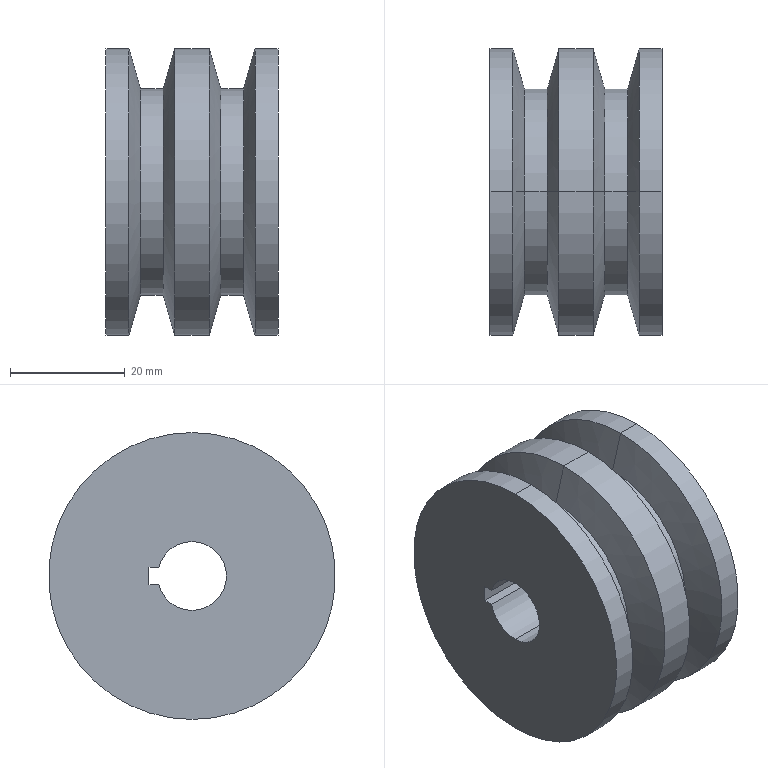Part | NX | features BREP 1 | 1 solid | 26 faces | box 30 x 50 x 50 mm | volume 43819 mm3 | cylinder 13 | cone 8 | plane 5 | commonest cylinder face diameters 50 x6 36 x4 12 x3
STEP:
#1=CARTESIAN_POINT('',(10.,0.,18.));
#2=VERTEX_POINT('',#1);
#3=CARTESIAN_POINT('',(10.,0.,-18.));
#4=VERTEX_POINT('',#3);
#5=CARTESIAN_POINT('',(10.,0.,0.));
#6=DIRECTION('',(-1.,0.,0.));
#7=DIRECTION('',(0.,0.,1.));
#8=AXIS2_PLACEMENT_3D('',#5,#6,#7);
#9=CIRCLE('',#8,18.);
#10=EDGE_CURVE('',#2,#4,#9,.T.);
#11=ORIENTED_EDGE('',*,*,#10,.T.);
#12=CARTESIAN_POINT('',(6.,0.,-18.));
#13=VERTEX_POINT('',#12);
#14=CARTESIAN_POINT('',(0.,0.,-18.));
#15=DIRECTION('',(-1.,0.,0.));
#16=VECTOR('',#15,1000.);
#17=LINE('',#14,#16);
#18=EDGE_CURVE('',#4,#13,#17,.T.);
#19=ORIENTED_EDGE('',*,*,#18,.T.);
#20=CARTESIAN_POINT('',(6.,0.,18.));
#21=VERTEX_POINT('',#20);
#22=CARTESIAN_POINT('',(6.,0.,0.));
#23=DIRECTION('',(-1.,0.,0.));
#24=DIRECTION('',(0.,0.,1.));
#25=AXIS2_PLACEMENT_3D('',#22,#23,#24);
#26=CIRCLE('',#25,18.);
#27=EDGE_CURVE('',#21,#13,#26,.T.);
#28=ORIENTED_EDGE('',*,*,#27,.F.);
#29=CARTESIAN_POINT('',(0.,0.,18.));
#30=DIRECTION('',(-1.,0.,0.));
#31=VECTOR('',#30,1000.);
#32=LINE('',#29,#31);
#33=EDGE_CURVE('',#2,#21,#32,.T.);
#34=ORIENTED_EDGE('',*,*,#33,.F.);
#35=EDGE_LOOP('',(#11,#19,#28,#34));
#36=FACE_BOUND('',#35,.T.);
#37=CARTESIAN_POINT('',(0.,0.,0.));
#38=DIRECTION('',(-1.,0.,0.));
#39=DIRECTION('',(0.,0.,-1.));
#40=AXIS2_PLACEMENT_3D('',#37,#38,#39);
#41=CYLINDRICAL_SURFACE('',#40,18.);
#42=ADVANCED_FACE('',(#36),#41,.T.);
#43=ORIENTED_EDGE('',*,*,#10,.F.);
#44=CARTESIAN_POINT('',(12.,0.,25.));
#45=VERTEX_POINT('',#44);
#46=CARTESIAN_POINT('',(12.,0.,25.));
#47=DIRECTION('',(0.2747,0.,0.9615));
#48=VECTOR('',#47,1000.);
#49=LINE('',#46,#48);
#50=EDGE_CURVE('',#45,#2,#49,.F.);
#51=ORIENTED_EDGE('',*,*,#50,.F.);
#52=CARTESIAN_POINT('',(12.,0.,-25.));
#53=VERTEX_POINT('',#52);
#54=CARTESIAN_POINT('',(12.,0.,0.));
#55=DIRECTION('',(-1.,0.,0.));
#56=DIRECTION('',(0.,0.,1.));
#57=AXIS2_PLACEMENT_3D('',#54,#55,#56);
#58=CIRCLE('',#57,25.);
#59=EDGE_CURVE('',#45,#53,#58,.T.);
#60=ORIENTED_EDGE('',*,*,#59,.T.);
#61=CARTESIAN_POINT('',(12.,0.,-25.));
#62=DIRECTION('',(0.2747,0.,-0.9615));
#63=VECTOR('',#62,1000.);
#64=LINE('',#61,#63);
#65=EDGE_CURVE('',#53,#4,#64,.F.);
#66=ORIENTED_EDGE('',*,*,#65,.T.);
#67=EDGE_LOOP('',(#43,#51,#60,#66));
#68=FACE_BOUND('',#67,.T.);
#69=CARTESIAN_POINT('',(12.,0.,0.));
#70=DIRECTION('',(1.,0.,0.));
#71=DIRECTION('',(0.,0.,1.));
#72=AXIS2_PLACEMENT_3D('',#69,#70,#71);
#73=CONICAL_SURFACE('',#72,25.,1.292);
#74=ADVANCED_FACE('',(#68),#73,.T.);
#75=CARTESIAN_POINT('',(18.,0.,25.));
#76=VERTEX_POINT('',#75);
#77=CARTESIAN_POINT('',(18.,0.,-25.));
#78=VERTEX_POINT('',#77);
#79=CARTESIAN_POINT('',(18.,0.,0.));
#80=DIRECTION('',(-1.,0.,0.));
#81=DIRECTION('',(0.,0.,1.));
#82=AXIS2_PLACEMENT_3D('',#79,#80,#81);
#83=CIRCLE('',#82,25.);
#84=EDGE_CURVE('',#76,#78,#83,.T.);
#85=ORIENTED_EDGE('',*,*,#84,.T.);
#86=CARTESIAN_POINT('',(0.,0.,-25.));
#87=DIRECTION('',(-1.,0.,0.));
#88=VECTOR('',#87,1000.);
#89=LINE('',#86,#88);
#90=EDGE_CURVE('',#78,#53,#89,.T.);
#91=ORIENTED_EDGE('',*,*,#90,.T.);
#92=ORIENTED_EDGE('',*,*,#59,.F.);
#93=CARTESIAN_POINT('',(0.,0.,25.));
#94=DIRECTION('',(-1.,0.,0.));
#95=VECTOR('',#94,1000.);
#96=LINE('',#93,#95);
#97=EDGE_CURVE('',#76,#45,#96,.T.);
#98=ORIENTED_EDGE('',*,*,#97,.F.);
#99=EDGE_LOOP('',(#85,#91,#92,#98));
#100=FACE_BOUND('',#99,.T.);
#101=CARTESIAN_POINT('',(0.,0.,0.));
#102=DIRECTION('',(-1.,0.,0.));
#103=DIRECTION('',(0.,0.,-1.));
#104=AXIS2_PLACEMENT_3D('',#101,#102,#103);
#105=CYLINDRICAL_SURFACE('',#104,25.);
#106=ADVANCED_FACE('',(#100),#105,.T.);
#107=CARTESIAN_POINT('',(20.,0.,18.));
#108=VERTEX_POINT('',#107);
#109=CARTESIAN_POINT('',(20.,0.,-18.));
#110=VERTEX_POINT('',#109);
#111=CARTESIAN_POINT('',(20.,0.,0.));
#112=DIRECTION('',(-1.,0.,0.));
#113=DIRECTION('',(0.,0.,1.));
#114=AXIS2_PLACEMENT_3D('',#111,#112,#113);
#115=CIRCLE('',#114,18.);
#116=EDGE_CURVE('',#108,#110,#115,.T.);
#117=ORIENTED_EDGE('',*,*,#116,.T.);
#118=CARTESIAN_POINT('',(20.,0.,-18.));
#119=DIRECTION('',(-0.2747,0.,-0.9615));
#120=VECTOR('',#119,1000.);
#121=LINE('',#118,#120);
#122=EDGE_CURVE('',#110,#78,#121,.T.);
#123=ORIENTED_EDGE('',*,*,#122,.T.);
#124=ORIENTED_EDGE('',*,*,#84,.F.);
#125=CARTESIAN_POINT('',(20.,0.,18.));
#126=DIRECTION('',(-0.2747,0.,0.9615));
#127=VECTOR('',#126,1000.);
#128=LINE('',#125,#127);
#129=EDGE_CURVE('',#108,#76,#128,.T.);
#130=ORIENTED_EDGE('',*,*,#129,.F.);
#131=EDGE_LOOP('',(#117,#123,#124,#130));
#132=FACE_BOUND('',#131,.T.);
#133=CARTESIAN_POINT('',(20.,0.,0.));
#134=DIRECTION('',(-1.,0.,0.));
#135=DIRECTION('',(0.,0.,-1.));
#136=AXIS2_PLACEMENT_3D('',#133,#134,#135);
#137=CONICAL_SURFACE('',#136,18.,1.292);
#138=ADVANCED_FACE('',(#132),#137,.T.);
#139=CARTESIAN_POINT('',(24.,0.,18.));
#140=VERTEX_POINT('',#139);
#141=CARTESIAN_POINT('',(24.,0.,-18.));
#142=VERTEX_POINT('',#141);
#143=CARTESIAN_POINT('',(24.,0.,0.));
#144=DIRECTION('',(-1.,0.,0.));
#145=DIRECTION('',(0.,0.,1.));
#146=AXIS2_PLACEMENT_3D('',#143,#144,#145);
#147=CIRCLE('',#146,18.);
#148=EDGE_CURVE('',#140,#142,#147,.T.);
#149=ORIENTED_EDGE('',*,*,#148,.T.);
#150=CARTESIAN_POINT('',(0.,0.,-18.));
#151=DIRECTION('',(-1.,0.,0.));
#152=VECTOR('',#151,1000.);
#153=LINE('',#150,#152);
#154=EDGE_CURVE('',#142,#110,#153,.T.);
#155=ORIENTED_EDGE('',*,*,#154,.T.);
#156=ORIENTED_EDGE('',*,*,#116,.F.);
#157=CARTESIAN_POINT('',(0.,0.,18.));
#158=DIRECTION('',(-1.,0.,0.));
#159=VECTOR('',#158,1000.);
#160=LINE('',#157,#159);
#161=EDGE_CURVE('',#140,#108,#160,.T.);
#162=ORIENTED_EDGE('',*,*,#161,.F.);
#163=EDGE_LOOP('',(#149,#155,#156,#162));
#164=FACE_BOUND('',#163,.T.);
#165=CARTESIAN_POINT('',(0.,0.,0.));
#166=DIRECTION('',(-1.,0.,0.));
#167=DIRECTION('',(0.,0.,-1.));
#168=AXIS2_PLACEMENT_3D('',#165,#166,#167);
#169=CYLINDRICAL_SURFACE('',#168,18.);
#170=ADVANCED_FACE('',(#164),#169,.T.);
#171=ORIENTED_EDGE('',*,*,#148,.F.);
#172=CARTESIAN_POINT('',(26.,0.,25.));
#173=VERTEX_POINT('',#172);
#174=CARTESIAN_POINT('',(26.,0.,25.));
#175=DIRECTION('',(0.2747,0.,0.9615));
#176=VECTOR('',#175,1000.);
#177=LINE('',#174,#176);
#178=EDGE_CURVE('',#173,#140,#177,.F.);
#179=ORIENTED_EDGE('',*,*,#178,.F.);
#180=CARTESIAN_POINT('',(26.,0.,-25.));
#181=VERTEX_POINT('',#180);
#182=CARTESIAN_POINT('',(26.,0.,0.));
#183=DIRECTION('',(-1.,0.,0.));
#184=DIRECTION('',(0.,0.,1.));
#185=AXIS2_PLACEMENT_3D('',#182,#183,#184);
#186=CIRCLE('',#185,25.);
#187=EDGE_CURVE('',#173,#181,#186,.T.);
#188=ORIENTED_EDGE('',*,*,#187,.T.);
#189=CARTESIAN_POINT('',(26.,0.,-25.));
#190=DIRECTION('',(0.2747,0.,-0.9615));
#191=VECTOR('',#190,1000.);
#192=LINE('',#189,#191);
#193=EDGE_CURVE('',#181,#142,#192,.F.);
#194=ORIENTED_EDGE('',*,*,#193,.T.);
#195=EDGE_LOOP('',(#171,#179,#188,#194));
#196=FACE_BOUND('',#195,.T.);
#197=CARTESIAN_POINT('',(26.,0.,0.));
#198=DIRECTION('',(1.,0.,0.));
#199=DIRECTION('',(0.,0.,1.));
#200=AXIS2_PLACEMENT_3D('',#197,#198,#199);
#201=CONICAL_SURFACE('',#200,25.,1.292);
#202=ADVANCED_FACE('',(#196),#201,.T.);
#203=CARTESIAN_POINT('',(30.,0.,25.));
#204=VERTEX_POINT('',#203);
#205=CARTESIAN_POINT('',(30.,0.,-25.));
#206=VERTEX_POINT('',#205);
#207=CARTESIAN_POINT('',(30.,0.,0.));
#208=DIRECTION('',(-1.,0.,0.));
#209=DIRECTION('',(0.,0.,1.));
#210=AXIS2_PLACEMENT_3D('',#207,#208,#209);
#211=CIRCLE('',#210,25.);
#212=EDGE_CURVE('',#204,#206,#211,.T.);
#213=ORIENTED_EDGE('',*,*,#212,.T.);
#214=CARTESIAN_POINT('',(0.,0.,-25.));
#215=DIRECTION('',(-1.,0.,0.));
#216=VECTOR('',#215,1000.);
#217=LINE('',#214,#216);
#218=EDGE_CURVE('',#206,#181,#217,.T.);
#219=ORIENTED_EDGE('',*,*,#218,.T.);
#220=ORIENTED_EDGE('',*,*,#187,.F.);
#221=CARTESIAN_POINT('',(0.,0.,25.));
#222=DIRECTION('',(-1.,0.,0.));
#223=VECTOR('',#222,1000.);
#224=LINE('',#221,#223);
#225=EDGE_CURVE('',#204,#173,#224,.T.);
#226=ORIENTED_EDGE('',*,*,#225,.F.);
#227=EDGE_LOOP('',(#213,#219,#220,#226));
#228=FACE_BOUND('',#227,.T.);
#229=CARTESIAN_POINT('',(0.,0.,0.));
#230=DIRECTION('',(-1.,0.,0.));
#231=DIRECTION('',(0.,0.,-1.));
#232=AXIS2_PLACEMENT_3D('',#229,#230,#231);
#233=CYLINDRICAL_SURFACE('',#232,25.);
#234=ADVANCED_FACE('',(#228),#233,.T.);
#235=CARTESIAN_POINT('',(30.,0.,-6.));
#236=VERTEX_POINT('',#235);
#237=CARTESIAN_POINT('',(30.,0.,6.));
#238=VERTEX_POINT('',#237);
#239=CARTESIAN_POINT('',(30.,0.,0.));
#240=DIRECTION('',(-1.,0.,0.));
#241=DIRECTION('',(0.,0.,1.));
#242=AXIS2_PLACEMENT_3D('',#239,#240,#241);
#243=CIRCLE('',#242,6.);
#244=EDGE_CURVE('',#236,#238,#243,.T.);
#245=ORIENTED_EDGE('',*,*,#244,.F.);
#246=CARTESIAN_POINT('',(0.,0.,-6.));
#247=VERTEX_POINT('',#246);
#248=CARTESIAN_POINT('',(0.,0.,-6.));
#249=DIRECTION('',(-1.,0.,0.));
#250=VECTOR('',#249,1000.);
#251=LINE('',#248,#250);
#252=EDGE_CURVE('',#236,#247,#251,.T.);
#253=ORIENTED_EDGE('',*,*,#252,.T.);
#254=CARTESIAN_POINT('',(0.,0.,6.));
#255=VERTEX_POINT('',#254);
#256=CARTESIAN_POINT('',(0.,0.,0.));
#257=DIRECTION('',(-1.,0.,0.));
#258=DIRECTION('',(0.,0.,1.));
#259=AXIS2_PLACEMENT_3D('',#256,#257,#258);
#260=CIRCLE('',#259,6.);
#261=EDGE_CURVE('',#247,#255,#260,.T.);
#262=ORIENTED_EDGE('',*,*,#261,.T.);
#263=CARTESIAN_POINT('',(0.,0.,6.));
#264=DIRECTION('',(-1.,0.,0.));
#265=VECTOR('',#264,1000.);
#266=LINE('',#263,#265);
#267=EDGE_CURVE('',#238,#255,#266,.T.);
#268=ORIENTED_EDGE('',*,*,#267,.F.);
#269=EDGE_LOOP('',(#245,#253,#262,#268));
#270=FACE_BOUND('',#269,.T.);
#271=CARTESIAN_POINT('',(0.,0.,0.));
#272=DIRECTION('',(-1.,0.,0.));
#273=DIRECTION('',(0.,0.,-1.));
#274=AXIS2_PLACEMENT_3D('',#271,#272,#273);
#275=CYLINDRICAL_SURFACE('',#274,6.);
#276=ADVANCED_FACE('',(#270),#275,.F.);
#277=CARTESIAN_POINT('',(30.,5.809,1.5));
#278=VERTEX_POINT('',#277);
#279=CARTESIAN_POINT('',(30.,0.,0.));
#280=DIRECTION('',(-1.,0.,0.));
#281=DIRECTION('',(0.,0.,1.));
#282=AXIS2_PLACEMENT_3D('',#279,#280,#281);
#283=CIRCLE('',#282,6.);
#284=EDGE_CURVE('',#238,#278,#283,.T.);
#285=ORIENTED_EDGE('',*,*,#284,.F.);
#286=ORIENTED_EDGE('',*,*,#267,.T.);
#287=CARTESIAN_POINT('',(0.,5.809,1.5));
#288=VERTEX_POINT('',#287);
#289=CARTESIAN_POINT('',(0.,0.,0.));
#290=DIRECTION('',(-1.,0.,0.));
#291=DIRECTION('',(0.,0.,1.));
#292=AXIS2_PLACEMENT_3D('',#289,#290,#291);
#293=CIRCLE('',#292,6.);
#294=EDGE_CURVE('',#255,#288,#293,.T.);
#295=ORIENTED_EDGE('',*,*,#294,.T.);
#296=CARTESIAN_POINT('',(30.,5.809,1.5));
#297=DIRECTION('',(-1.,0.,0.));
#298=VECTOR('',#297,1000.);
#299=LINE('',#296,#298);
#300=EDGE_CURVE('',#278,#288,#299,.T.);
#301=ORIENTED_EDGE('',*,*,#300,.F.);
#302=EDGE_LOOP('',(#285,#286,#295,#301));
#303=FACE_BOUND('',#302,.T.);
#304=CARTESIAN_POINT('',(0.,0.,0.));
#305=DIRECTION('',(-1.,0.,0.));
#306=DIRECTION('',(0.,0.,-1.));
#307=AXIS2_PLACEMENT_3D('',#304,#305,#306);
#308=CYLINDRICAL_SURFACE('',#307,6.);
#309=ADVANCED_FACE('',(#303),#308,.F.);
#310=CARTESIAN_POINT('',(4.,0.,25.));
#311=VERTEX_POINT('',#310);
#312=CARTESIAN_POINT('',(4.,0.,-25.));
#313=VERTEX_POINT('',#312);
#314=CARTESIAN_POINT('',(4.,0.,0.));
#315=DIRECTION('',(-1.,0.,0.));
#316=DIRECTION('',(0.,0.,1.));
#317=AXIS2_PLACEMENT_3D('',#314,#315,#316);
#318=CIRCLE('',#317,25.);
#319=EDGE_CURVE('',#311,#313,#318,.T.);
#320=ORIENTED_EDGE('',*,*,#319,.T.);
#321=CARTESIAN_POINT('',(0.,0.,-25.));
#322=VERTEX_POINT('',#321);
#323=CARTESIAN_POINT('',(0.,0.,-25.));
#324=DIRECTION('',(-1.,0.,0.));
#325=VECTOR('',#324,1000.);
#326=LINE('',#323,#325);
#327=EDGE_CURVE('',#313,#322,#326,.T.);
#328=ORIENTED_EDGE('',*,*,#327,.T.);
#329=CARTESIAN_POINT('',(0.,0.,25.));
#330=VERTEX_POINT('',#329);
#331=CARTESIAN_POINT('',(0.,0.,0.));
#332=DIRECTION('',(-1.,0.,0.));
#333=DIRECTION('',(0.,0.,1.));
#334=AXIS2_PLACEMENT_3D('',#331,#332,#333);
#335=CIRCLE('',#334,25.);
#336=EDGE_CURVE('',#330,#322,#335,.T.);
#337=ORIENTED_EDGE('',*,*,#336,.F.);
#338=CARTESIAN_POINT('',(0.,0.,25.));
#339=DIRECTION('',(-1.,0.,0.));
#340=VECTOR('',#339,1000.);
#341=LINE('',#338,#340);
#342=EDGE_CURVE('',#311,#330,#341,.T.);
#343=ORIENTED_EDGE('',*,*,#342,.F.);
#344=EDGE_LOOP('',(#320,#328,#337,#343));
#345=FACE_BOUND('',#344,.T.);
#346=CARTESIAN_POINT('',(0.,0.,0.));
#347=DIRECTION('',(-1.,0.,0.));
#348=DIRECTION('',(0.,0.,-1.));
#349=AXIS2_PLACEMENT_3D('',#346,#347,#348);
#350=CYLINDRICAL_SURFACE('',#349,25.);
#351=ADVANCED_FACE('',(#345),#350,.T.);
#352=ORIENTED_EDGE('',*,*,#27,.T.);
#353=CARTESIAN_POINT('',(6.,0.,-18.));
#354=DIRECTION('',(-0.2747,0.,-0.9615));
#355=VECTOR('',#354,1000.);
#356=LINE('',#353,#355);
#357=EDGE_CURVE('',#13,#313,#356,.T.);
#358=ORIENTED_EDGE('',*,*,#357,.T.);
#359=ORIENTED_EDGE('',*,*,#319,.F.);
#360=CARTESIAN_POINT('',(6.,0.,18.));
#361=DIRECTION('',(-0.2747,0.,0.9615));
#362=VECTOR('',#361,1000.);
#363=LINE('',#360,#362);
#364=EDGE_CURVE('',#21,#311,#363,.T.);
#365=ORIENTED_EDGE('',*,*,#364,.F.);
#366=EDGE_LOOP('',(#352,#358,#359,#365));
#367=FACE_BOUND('',#366,.T.);
#368=CARTESIAN_POINT('',(6.,0.,0.));
#369=DIRECTION('',(-1.,0.,0.));
#370=DIRECTION('',(0.,0.,-1.));
#371=AXIS2_PLACEMENT_3D('',#368,#369,#370);
#372=CONICAL_SURFACE('',#371,18.,1.292);
#373=ADVANCED_FACE('',(#367),#372,.T.);
#374=ORIENTED_EDGE('',*,*,#357,.F.);
#375=CARTESIAN_POINT('',(6.,0.,0.));
#376=DIRECTION('',(-1.,0.,0.));
#377=DIRECTION('',(0.,0.,1.));
#378=AXIS2_PLACEMENT_3D('',#375,#376,#377);
#379=CIRCLE('',#378,18.);
#380=EDGE_CURVE('',#13,#21,#379,.T.);
#381=ORIENTED_EDGE('',*,*,#380,.T.);
#382=ORIENTED_EDGE('',*,*,#364,.T.);
#383=CARTESIAN_POINT('',(4.,0.,0.));
#384=DIRECTION('',(-1.,0.,0.));
#385=DIRECTION('',(0.,0.,1.));
#386=AXIS2_PLACEMENT_3D('',#383,#384,#385);
#387=CIRCLE('',#386,25.);
#388=EDGE_CURVE('',#313,#311,#387,.T.);
#389=ORIENTED_EDGE('',*,*,#388,.F.);
#390=EDGE_LOOP('',(#374,#381,#382,#389));
#391=FACE_BOUND('',#390,.T.);
#392=CARTESIAN_POINT('',(6.,0.,0.));
#393=DIRECTION('',(-1.,0.,0.));
#394=DIRECTION('',(0.,0.,-1.));
#395=AXIS2_PLACEMENT_3D('',#392,#393,#394);
#396=CONICAL_SURFACE('',#395,18.,1.292);
#397=ADVANCED_FACE('',(#391),#396,.T.);
#398=ORIENTED_EDGE('',*,*,#327,.F.);
#399=ORIENTED_EDGE('',*,*,#388,.T.);
#400=ORIENTED_EDGE('',*,*,#342,.T.);
#401=CARTESIAN_POINT('',(0.,0.,0.));
#402=DIRECTION('',(-1.,0.,0.));
#403=DIRECTION('',(0.,0.,1.));
#404=AXIS2_PLACEMENT_3D('',#401,#402,#403);
#405=CIRCLE('',#404,25.);
#406=EDGE_CURVE('',#322,#330,#405,.T.);
#407=ORIENTED_EDGE('',*,*,#406,.F.);
#408=EDGE_LOOP('',(#398,#399,#400,#407));
#409=FACE_BOUND('',#408,.T.);
#410=CARTESIAN_POINT('',(0.,0.,0.));
#411=DIRECTION('',(-1.,0.,0.));
#412=DIRECTION('',(0.,0.,-1.));
#413=AXIS2_PLACEMENT_3D('',#410,#411,#412);
#414=CYLINDRICAL_SURFACE('',#413,25.);
#415=ADVANCED_FACE('',(#409),#414,.T.);
#416=ORIENTED_EDGE('',*,*,#336,.T.);
#417=ORIENTED_EDGE('',*,*,#406,.T.);
#418=EDGE_LOOP('',(#416,#417));
#419=FACE_BOUND('',#418,.T.);
#420=CARTESIAN_POINT('',(0.,7.5,1.5));
#421=VERTEX_POINT('',#420);
#422=CARTESIAN_POINT('',(0.,7.5,-1.5));
#423=VERTEX_POINT('',#422);
#424=CARTESIAN_POINT('',(0.,7.5,-1.5));
#425=DIRECTION('',(0.,0.,-1.));
#426=VECTOR('',#425,1000.);
#427=LINE('',#424,#426);
#428=EDGE_CURVE('',#421,#423,#427,.T.);
#429=ORIENTED_EDGE('',*,*,#428,.F.);
#430=CARTESIAN_POINT('',(0.,5.809,1.5));
#431=DIRECTION('',(0.,1.,0.));
#432=VECTOR('',#431,1000.);
#433=LINE('',#430,#432);
#434=EDGE_CURVE('',#288,#421,#433,.T.);
#435=ORIENTED_EDGE('',*,*,#434,.F.);
#436=ORIENTED_EDGE('',*,*,#294,.F.);
#437=ORIENTED_EDGE('',*,*,#261,.F.);
#438=CARTESIAN_POINT('',(0.,5.809,-1.5));
#439=VERTEX_POINT('',#438);
#440=CARTESIAN_POINT('',(0.,0.,0.));
#441=DIRECTION('',(-1.,0.,0.));
#442=DIRECTION('',(0.,0.,1.));
#443=AXIS2_PLACEMENT_3D('',#440,#441,#442);
#444=CIRCLE('',#443,6.);
#445=EDGE_CURVE('',#439,#247,#444,.T.);
#446=ORIENTED_EDGE('',*,*,#445,.F.);
#447=CARTESIAN_POINT('',(0.,5.809,-1.5));
#448=DIRECTION('',(0.,-1.,0.));
#449=VECTOR('',#448,1000.);
#450=LINE('',#447,#449);
#451=EDGE_CURVE('',#423,#439,#450,.T.);
#452=ORIENTED_EDGE('',*,*,#451,.F.);
#453=EDGE_LOOP('',(#429,#435,#436,#437,#446,#452));
#454=FACE_BOUND('',#453,.T.);
#455=CARTESIAN_POINT('',(0.,6.,0.));
#456=DIRECTION('',(1.,0.,0.));
#457=DIRECTION('',(0.,1.,0.));
#458=AXIS2_PLACEMENT_3D('',#455,#456,#457);
#459=PLANE('',#458);
#460=ADVANCED_FACE('',(#419,#454),#459,.F.);
#461=ORIENTED_EDGE('',*,*,#252,.F.);
#462=CARTESIAN_POINT('',(30.,5.809,-1.5));
#463=VERTEX_POINT('',#462);
#464=CARTESIAN_POINT('',(30.,0.,0.));
#465=DIRECTION('',(-1.,0.,0.));
#466=DIRECTION('',(0.,0.,1.));
#467=AXIS2_PLACEMENT_3D('',#464,#465,#466);
#468=CIRCLE('',#467,6.);
#469=EDGE_CURVE('',#463,#236,#468,.T.);
#470=ORIENTED_EDGE('',*,*,#469,.F.);
#471=CARTESIAN_POINT('',(30.,5.809,-1.5));
#472=DIRECTION('',(-1.,0.,0.));
#473=VECTOR('',#472,1000.);
#474=LINE('',#471,#473);
#475=EDGE_CURVE('',#463,#439,#474,.T.);
#476=ORIENTED_EDGE('',*,*,#475,.T.);
#477=ORIENTED_EDGE('',*,*,#445,.T.);
#478=EDGE_LOOP('',(#461,#470,#476,#477));
#479=FACE_BOUND('',#478,.T.);
#480=CARTESIAN_POINT('',(0.,0.,0.));
#481=DIRECTION('',(-1.,0.,0.));
#482=DIRECTION('',(0.,0.,-1.));
#483=AXIS2_PLACEMENT_3D('',#480,#481,#482);
#484=CYLINDRICAL_SURFACE('',#483,6.);
#485=ADVANCED_FACE('',(#479),#484,.F.);
#486=ORIENTED_EDGE('',*,*,#212,.F.);
#487=CARTESIAN_POINT('',(30.,0.,0.));
#488=DIRECTION('',(-1.,0.,0.));
#489=DIRECTION('',(0.,0.,1.));
#490=AXIS2_PLACEMENT_3D('',#487,#488,#489);
#491=CIRCLE('',#490,25.);
#492=EDGE_CURVE('',#206,#204,#491,.T.);
#493=ORIENTED_EDGE('',*,*,#492,.F.);
#494=EDGE_LOOP('',(#486,#493));
#495=FACE_BOUND('',#494,.T.);
#496=ORIENTED_EDGE('',*,*,#469,.T.);
#497=ORIENTED_EDGE('',*,*,#244,.T.);
#498=ORIENTED_EDGE('',*,*,#284,.T.);
#499=CARTESIAN_POINT('',(30.,7.5,1.5));
#500=VERTEX_POINT('',#499);
#501=CARTESIAN_POINT('',(30.,5.809,1.5));
#502=DIRECTION('',(0.,1.,0.));
#503=VECTOR('',#502,1000.);
#504=LINE('',#501,#503);
#505=EDGE_CURVE('',#278,#500,#504,.T.);
#506=ORIENTED_EDGE('',*,*,#505,.T.);
#507=CARTESIAN_POINT('',(30.,7.5,-1.5));
#508=VERTEX_POINT('',#507);
#509=CARTESIAN_POINT('',(30.,7.5,-1.5));
#510=DIRECTION('',(0.,0.,-1.));
#511=VECTOR('',#510,1000.);
#512=LINE('',#509,#511);
#513=EDGE_CURVE('',#500,#508,#512,.T.);
#514=ORIENTED_EDGE('',*,*,#513,.T.);
#515=CARTESIAN_POINT('',(30.,5.809,-1.5));
#516=DIRECTION('',(0.,-1.,0.));
#517=VECTOR('',#516,1000.);
#518=LINE('',#515,#517);
#519=EDGE_CURVE('',#508,#463,#518,.T.);
#520=ORIENTED_EDGE('',*,*,#519,.T.);
#521=EDGE_LOOP('',(#496,#497,#498,#506,#514,#520));
#522=FACE_BOUND('',#521,.T.);
#523=CARTESIAN_POINT('',(30.,25.,0.));
#524=DIRECTION('',(-1.,0.,0.));
#525=DIRECTION('',(0.,0.,-1.));
#526=AXIS2_PLACEMENT_3D('',#523,#524,#525);
#527=PLANE('',#526);
#528=ADVANCED_FACE('',(#495,#522),#527,.F.);
#529=ORIENTED_EDGE('',*,*,#218,.F.);
#530=ORIENTED_EDGE('',*,*,#492,.T.);
#531=ORIENTED_EDGE('',*,*,#225,.T.);
#532=CARTESIAN_POINT('',(26.,0.,0.));
#533=DIRECTION('',(-1.,0.,0.));
#534=DIRECTION('',(0.,0.,1.));
#535=AXIS2_PLACEMENT_3D('',#532,#533,#534);
#536=CIRCLE('',#535,25.);
#537=EDGE_CURVE('',#181,#173,#536,.T.);
#538=ORIENTED_EDGE('',*,*,#537,.F.);
#539=EDGE_LOOP('',(#529,#530,#531,#538));
#540=FACE_BOUND('',#539,.T.);
#541=CARTESIAN_POINT('',(0.,0.,0.));
#542=DIRECTION('',(-1.,0.,0.));
#543=DIRECTION('',(0.,0.,-1.));
#544=AXIS2_PLACEMENT_3D('',#541,#542,#543);
#545=CYLINDRICAL_SURFACE('',#544,25.);
#546=ADVANCED_FACE('',(#540),#545,.T.);
#547=ORIENTED_EDGE('',*,*,#178,.T.);
#548=CARTESIAN_POINT('',(24.,0.,0.));
#549=DIRECTION('',(-1.,0.,0.));
#550=DIRECTION('',(0.,0.,1.));
#551=AXIS2_PLACEMENT_3D('',#548,#549,#550);
#552=CIRCLE('',#551,18.);
#553=EDGE_CURVE('',#142,#140,#552,.T.);
#554=ORIENTED_EDGE('',*,*,#553,.F.);
#555=ORIENTED_EDGE('',*,*,#193,.F.);
#556=ORIENTED_EDGE('',*,*,#537,.T.);
#557=EDGE_LOOP('',(#547,#554,#555,#556));
#558=FACE_BOUND('',#557,.T.);
#559=CARTESIAN_POINT('',(26.,0.,0.));
#560=DIRECTION('',(1.,0.,0.));
#561=DIRECTION('',(0.,0.,1.));
#562=AXIS2_PLACEMENT_3D('',#559,#560,#561);
#563=CONICAL_SURFACE('',#562,25.,1.292);
#564=ADVANCED_FACE('',(#558),#563,.T.);
#565=ORIENTED_EDGE('',*,*,#154,.F.);
#566=ORIENTED_EDGE('',*,*,#553,.T.);
#567=ORIENTED_EDGE('',*,*,#161,.T.);
#568=CARTESIAN_POINT('',(20.,0.,0.));
#569=DIRECTION('',(-1.,0.,0.));
#570=DIRECTION('',(0.,0.,1.));
#571=AXIS2_PLACEMENT_3D('',#568,#569,#570);
#572=CIRCLE('',#571,18.);
#573=EDGE_CURVE('',#110,#108,#572,.T.);
#574=ORIENTED_EDGE('',*,*,#573,.F.);
#575=EDGE_LOOP('',(#565,#566,#567,#574));
#576=FACE_BOUND('',#575,.T.);
#577=CARTESIAN_POINT('',(0.,0.,0.));
#578=DIRECTION('',(-1.,0.,0.));
#579=DIRECTION('',(0.,0.,-1.));
#580=AXIS2_PLACEMENT_3D('',#577,#578,#579);
#581=CYLINDRICAL_SURFACE('',#580,18.);
#582=ADVANCED_FACE('',(#576),#581,.T.);
#583=ORIENTED_EDGE('',*,*,#122,.F.);
#584=ORIENTED_EDGE('',*,*,#573,.T.);
#585=ORIENTED_EDGE('',*,*,#129,.T.);
#586=CARTESIAN_POINT('',(18.,0.,0.));
#587=DIRECTION('',(-1.,0.,0.));
#588=DIRECTION('',(0.,0.,1.));
#589=AXIS2_PLACEMENT_3D('',#586,#587,#588);
#590=CIRCLE('',#589,25.);
#591=EDGE_CURVE('',#78,#76,#590,.T.);
#592=ORIENTED_EDGE('',*,*,#591,.F.);
#593=EDGE_LOOP('',(#583,#584,#585,#592));
#594=FACE_BOUND('',#593,.T.);
#595=CARTESIAN_POINT('',(20.,0.,0.));
#596=DIRECTION('',(-1.,0.,0.));
#597=DIRECTION('',(0.,0.,-1.));
#598=AXIS2_PLACEMENT_3D('',#595,#596,#597);
#599=CONICAL_SURFACE('',#598,18.,1.292);
#600=ADVANCED_FACE('',(#594),#599,.T.);
#601=ORIENTED_EDGE('',*,*,#90,.F.);
#602=ORIENTED_EDGE('',*,*,#591,.T.);
#603=ORIENTED_EDGE('',*,*,#97,.T.);
#604=CARTESIAN_POINT('',(12.,0.,0.));
#605=DIRECTION('',(-1.,0.,0.));
#606=DIRECTION('',(0.,0.,1.));
#607=AXIS2_PLACEMENT_3D('',#604,#605,#606);
#608=CIRCLE('',#607,25.);
#609=EDGE_CURVE('',#53,#45,#608,.T.);
#610=ORIENTED_EDGE('',*,*,#609,.F.);
#611=EDGE_LOOP('',(#601,#602,#603,#610));
#612=FACE_BOUND('',#611,.T.);
#613=CARTESIAN_POINT('',(0.,0.,0.));
#614=DIRECTION('',(-1.,0.,0.));
#615=DIRECTION('',(0.,0.,-1.));
#616=AXIS2_PLACEMENT_3D('',#613,#614,#615);
#617=CYLINDRICAL_SURFACE('',#616,25.);
#618=ADVANCED_FACE('',(#612),#617,.T.);
#619=ORIENTED_EDGE('',*,*,#50,.T.);
#620=CARTESIAN_POINT('',(10.,0.,0.));
#621=DIRECTION('',(-1.,0.,0.));
#622=DIRECTION('',(0.,0.,1.));
#623=AXIS2_PLACEMENT_3D('',#620,#621,#622);
#624=CIRCLE('',#623,18.);
#625=EDGE_CURVE('',#4,#2,#624,.T.);
#626=ORIENTED_EDGE('',*,*,#625,.F.);
#627=ORIENTED_EDGE('',*,*,#65,.F.);
#628=ORIENTED_EDGE('',*,*,#609,.T.);
#629=EDGE_LOOP('',(#619,#626,#627,#628));
#630=FACE_BOUND('',#629,.T.);
#631=CARTESIAN_POINT('',(12.,0.,0.));
#632=DIRECTION('',(1.,0.,0.));
#633=DIRECTION('',(0.,0.,1.));
#634=AXIS2_PLACEMENT_3D('',#631,#632,#633);
#635=CONICAL_SURFACE('',#634,25.,1.292);
#636=ADVANCED_FACE('',(#630),#635,.T.);
#637=ORIENTED_EDGE('',*,*,#18,.F.);
#638=ORIENTED_EDGE('',*,*,#625,.T.);
#639=ORIENTED_EDGE('',*,*,#33,.T.);
#640=ORIENTED_EDGE('',*,*,#380,.F.);
#641=EDGE_LOOP('',(#637,#638,#639,#640));
#642=FACE_BOUND('',#641,.T.);
#643=CARTESIAN_POINT('',(0.,0.,0.));
#644=DIRECTION('',(-1.,0.,0.));
#645=DIRECTION('',(0.,0.,-1.));
#646=AXIS2_PLACEMENT_3D('',#643,#644,#645);
#647=CYLINDRICAL_SURFACE('',#646,18.);
#648=ADVANCED_FACE('',(#642),#647,.T.);
#649=ORIENTED_EDGE('',*,*,#428,.T.);
#650=CARTESIAN_POINT('',(30.,7.5,-1.5));
#651=DIRECTION('',(-1.,0.,0.));
#652=VECTOR('',#651,1000.);
#653=LINE('',#650,#652);
#654=EDGE_CURVE('',#508,#423,#653,.T.);
#655=ORIENTED_EDGE('',*,*,#654,.F.);
#656=ORIENTED_EDGE('',*,*,#513,.F.);
#657=CARTESIAN_POINT('',(30.,7.5,1.5));
#658=DIRECTION('',(-1.,0.,0.));
#659=VECTOR('',#658,1000.);
#660=LINE('',#657,#659);
#661=EDGE_CURVE('',#500,#421,#660,.T.);
#662=ORIENTED_EDGE('',*,*,#661,.T.);
#663=EDGE_LOOP('',(#649,#655,#656,#662));
#664=FACE_BOUND('',#663,.T.);
#665=CARTESIAN_POINT('',(30.,7.5,-1.5));
#666=DIRECTION('',(0.,1.,0.));
#667=DIRECTION('',(-1.,0.,0.));
#668=AXIS2_PLACEMENT_3D('',#665,#666,#667);
#669=PLANE('',#668);
#670=ADVANCED_FACE('',(#664),#669,.F.);
#671=ORIENTED_EDGE('',*,*,#434,.T.);
#672=ORIENTED_EDGE('',*,*,#661,.F.);
#673=ORIENTED_EDGE('',*,*,#505,.F.);
#674=ORIENTED_EDGE('',*,*,#300,.T.);
#675=EDGE_LOOP('',(#671,#672,#673,#674));
#676=FACE_BOUND('',#675,.T.);
#677=CARTESIAN_POINT('',(30.,5.809,1.5));
#678=DIRECTION('',(0.,0.,1.));
#679=DIRECTION('',(0.,1.,0.));
#680=AXIS2_PLACEMENT_3D('',#677,#678,#679);
#681=PLANE('',#680);
#682=ADVANCED_FACE('',(#676),#681,.F.);
#683=ORIENTED_EDGE('',*,*,#451,.T.);
#684=ORIENTED_EDGE('',*,*,#475,.F.);
#685=ORIENTED_EDGE('',*,*,#519,.F.);
#686=ORIENTED_EDGE('',*,*,#654,.T.);
#687=EDGE_LOOP('',(#683,#684,#685,#686));
#688=FACE_BOUND('',#687,.T.);
#689=CARTESIAN_POINT('',(30.,5.809,-1.5));
#690=DIRECTION('',(0.,0.,-1.));
#691=DIRECTION('',(1.,0.,0.));
#692=AXIS2_PLACEMENT_3D('',#689,#690,#691);
#693=PLANE('',#692);
#694=ADVANCED_FACE('',(#688),#693,.F.);
#695=CLOSED_SHELL('',(#42,#74,#106,#138,#170,#202,#234,#276,#309,#351,#373,#397,#415,#460,#485,#528,#546,#564,#582,#600,#618,#636,#648,#670,#682,#694));
#696=MANIFOLD_SOLID_BREP('',#695);
#697=(LENGTH_UNIT()NAMED_UNIT(*)SI_UNIT(.MILLI.,.METRE.));
#698=UNCERTAINTY_MEASURE_WITH_UNIT(LENGTH_MEASURE(0.00001),#697,'','');
#699=(NAMED_UNIT(*)PLANE_ANGLE_UNIT()SI_UNIT($,.RADIAN.));
#700=(NAMED_UNIT(*)SI_UNIT($,.STERADIAN.)SOLID_ANGLE_UNIT());
#701=(GEOMETRIC_REPRESENTATION_CONTEXT(3)GLOBAL_UNCERTAINTY_ASSIGNED_CONTEXT((#698))GLOBAL_UNIT_ASSIGNED_CONTEXT((#697,#699,#700))REPRESENTATION_CONTEXT('',''));
#702=ADVANCED_BREP_SHAPE_REPRESENTATION('',(#696),#701);